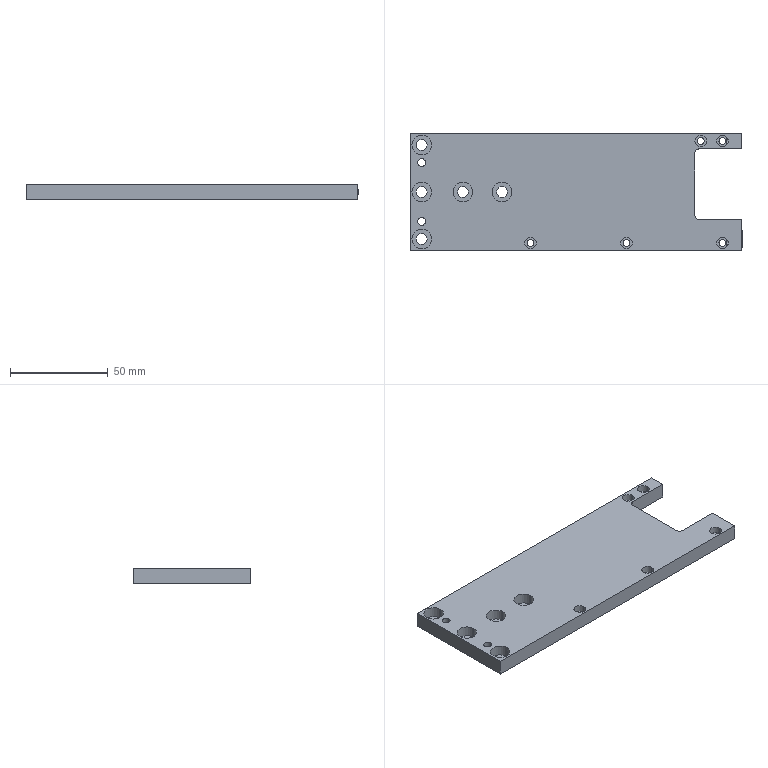Part | SolidWorks | features BaseBody 1 | 1 solid | 74 faces | box 169.5 x 60 x 8 mm | volume 71017 mm3 | cylinder 50 | plane 20 | cone 4 | commonest cylinder face diameters 3.5 x10 5.5 x10 6 x10 10 x10 4 x6 2.459 x4